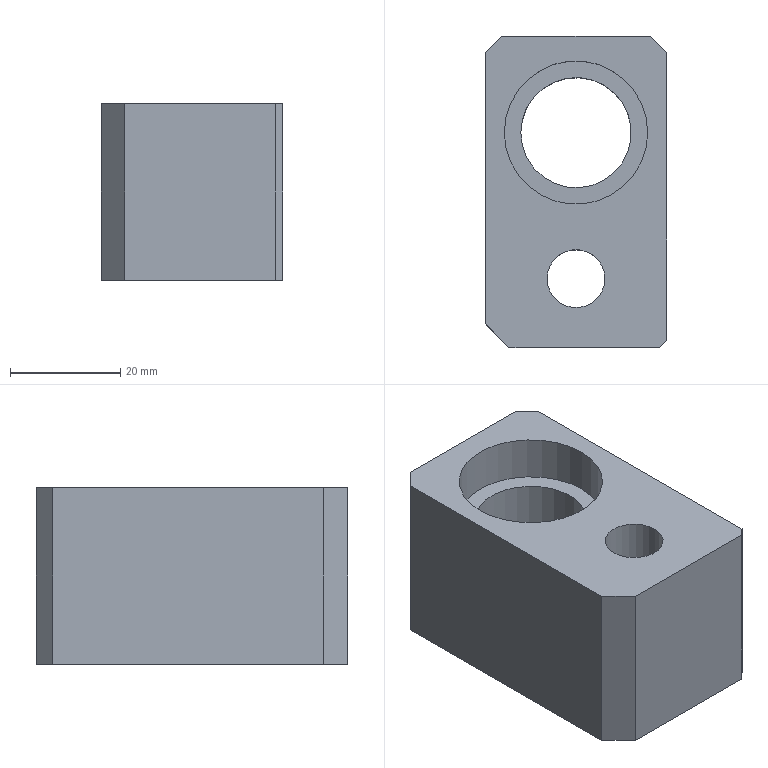Part | STEP file | lll_id2666_x_t | 1 solid | 16 faces | box 33 x 56.5 x 32 mm | volume 42057 mm3 | plane 12 | cylinder 4 | commonest cylinder face diameters 10.5 x1 17 x1 20 x1 26 x1
STEP:
#1=CARTESIAN_POINT('',(427.,300.,60.5));
#2=VERTEX_POINT('',#1);
#3=CARTESIAN_POINT('',(437.,300.,60.5));
#4=DIRECTION('',(0.,0.,1.));
#5=DIRECTION('',(-1.,0.,0.));
#6=AXIS2_PLACEMENT_3D('',#3,#4,#5);
#7=CIRCLE('',#6,10.);
#8=EDGE_CURVE('',#2,#2,#7,.T.);
#9=ORIENTED_EDGE('',*,*,#8,.T.);
#10=EDGE_LOOP('',(#9));
#11=FACE_BOUND('',#10,.T.);
#12=CARTESIAN_POINT('',(450.5,317.5,60.5));
#13=VERTEX_POINT('',#12);
#14=CARTESIAN_POINT('',(423.5,317.5,60.5));
#15=VERTEX_POINT('',#14);
#16=CARTESIAN_POINT('',(437.,317.5,60.5));
#17=DIRECTION('',(-1.,0.,0.));
#18=VECTOR('',#17,1.);
#19=LINE('',#16,#18);
#20=EDGE_CURVE('',#13,#15,#19,.T.);
#21=ORIENTED_EDGE('',*,*,#20,.F.);
#22=CARTESIAN_POINT('',(453.5,314.5,60.5));
#23=VERTEX_POINT('',#22);
#24=CARTESIAN_POINT('',(434.043,333.957,60.5));
#25=DIRECTION('',(0.7071,-0.7071,0.));
#26=VECTOR('',#25,1.);
#27=LINE('',#24,#26);
#28=EDGE_CURVE('',#13,#23,#27,.T.);
#29=ORIENTED_EDGE('',*,*,#28,.T.);
#30=CARTESIAN_POINT('',(453.5,262.343,60.5));
#31=VERTEX_POINT('',#30);
#32=CARTESIAN_POINT('',(453.5,300.,60.5));
#33=DIRECTION('',(0.,1.,0.));
#34=VECTOR('',#33,1.);
#35=LINE('',#32,#34);
#36=EDGE_CURVE('',#31,#23,#35,.T.);
#37=ORIENTED_EDGE('',*,*,#36,.F.);
#38=CARTESIAN_POINT('',(452.157,261.,60.5));
#39=VERTEX_POINT('',#38);
#40=CARTESIAN_POINT('',(409.396,218.239,60.5));
#41=DIRECTION('',(-0.7071,-0.7071,0.));
#42=VECTOR('',#41,1.);
#43=LINE('',#40,#42);
#44=EDGE_CURVE('',#31,#39,#43,.T.);
#45=ORIENTED_EDGE('',*,*,#44,.T.);
#46=CARTESIAN_POINT('',(424.843,261.,60.5));
#47=VERTEX_POINT('',#46);
#48=CARTESIAN_POINT('',(437.,261.,60.5));
#49=DIRECTION('',(1.,0.,0.));
#50=VECTOR('',#49,1.);
#51=LINE('',#48,#50);
#52=EDGE_CURVE('',#47,#39,#51,.T.);
#53=ORIENTED_EDGE('',*,*,#52,.F.);
#54=CARTESIAN_POINT('',(420.5,265.343,60.5));
#55=VERTEX_POINT('',#54);
#56=CARTESIAN_POINT('',(397.964,287.879,60.5));
#57=DIRECTION('',(-0.7071,0.7071,0.));
#58=VECTOR('',#57,1.);
#59=LINE('',#56,#58);
#60=EDGE_CURVE('',#47,#55,#59,.T.);
#61=ORIENTED_EDGE('',*,*,#60,.T.);
#62=CARTESIAN_POINT('',(420.5,314.5,60.5));
#63=VERTEX_POINT('',#62);
#64=CARTESIAN_POINT('',(420.5,300.,60.5));
#65=DIRECTION('',(0.,-1.,0.));
#66=VECTOR('',#65,1.);
#67=LINE('',#64,#66);
#68=EDGE_CURVE('',#63,#55,#67,.T.);
#69=ORIENTED_EDGE('',*,*,#68,.F.);
#70=CARTESIAN_POINT('',(371.817,265.817,60.5));
#71=DIRECTION('',(0.7071,0.7071,0.));
#72=VECTOR('',#71,1.);
#73=LINE('',#70,#72);
#74=EDGE_CURVE('',#63,#15,#73,.T.);
#75=ORIENTED_EDGE('',*,*,#74,.T.);
#76=EDGE_LOOP('',(#21,#29,#37,#45,#53,#61,#69,#75));
#77=FACE_BOUND('',#76,.T.);
#78=CARTESIAN_POINT('',(445.5,273.5,60.5));
#79=VERTEX_POINT('',#78);
#80=CARTESIAN_POINT('',(437.,273.5,60.5));
#81=DIRECTION('',(0.,0.,1.));
#82=DIRECTION('',(1.,0.,0.));
#83=AXIS2_PLACEMENT_3D('',#80,#81,#82);
#84=CIRCLE('',#83,8.5);
#85=EDGE_CURVE('',#79,#79,#84,.T.);
#86=ORIENTED_EDGE('',*,*,#85,.T.);
#87=EDGE_LOOP('',(#86));
#88=FACE_BOUND('',#87,.T.);
#89=CARTESIAN_POINT('',(368.86,268.775,60.5));
#90=DIRECTION('',(0.,0.,1.));
#91=DIRECTION('',(-1.,0.,0.));
#92=AXIS2_PLACEMENT_3D('',#89,#90,#91);
#93=PLANE('',#92);
#94=ADVANCED_FACE('',(#11,#77,#88),#93,.F.);
#95=CARTESIAN_POINT('',(450.,300.,92.5));
#96=VERTEX_POINT('',#95);
#97=CARTESIAN_POINT('',(437.,300.,92.5));
#98=DIRECTION('',(0.,0.,1.));
#99=DIRECTION('',(1.,0.,0.));
#100=AXIS2_PLACEMENT_3D('',#97,#98,#99);
#101=CIRCLE('',#100,13.);
#102=EDGE_CURVE('',#96,#96,#101,.T.);
#103=ORIENTED_EDGE('',*,*,#102,.F.);
#104=EDGE_LOOP('',(#103));
#105=FACE_BOUND('',#104,.T.);
#106=CARTESIAN_POINT('',(442.25,273.5,92.5));
#107=VERTEX_POINT('',#106);
#108=CARTESIAN_POINT('',(437.,273.5,92.5));
#109=DIRECTION('',(0.,0.,1.));
#110=DIRECTION('',(1.,0.,0.));
#111=AXIS2_PLACEMENT_3D('',#108,#109,#110);
#112=CIRCLE('',#111,5.25);
#113=EDGE_CURVE('',#107,#107,#112,.T.);
#114=ORIENTED_EDGE('',*,*,#113,.F.);
#115=EDGE_LOOP('',(#114));
#116=FACE_BOUND('',#115,.T.);
#117=CARTESIAN_POINT('',(453.5,314.5,92.5));
#118=VERTEX_POINT('',#117);
#119=CARTESIAN_POINT('',(453.5,262.343,92.5));
#120=VERTEX_POINT('',#119);
#121=CARTESIAN_POINT('',(453.5,300.,92.5));
#122=DIRECTION('',(0.,-1.,0.));
#123=VECTOR('',#122,1.);
#124=LINE('',#121,#123);
#125=EDGE_CURVE('',#118,#120,#124,.T.);
#126=ORIENTED_EDGE('',*,*,#125,.F.);
#127=CARTESIAN_POINT('',(450.5,317.5,92.5));
#128=VERTEX_POINT('',#127);
#129=CARTESIAN_POINT('',(434.043,333.957,92.5));
#130=DIRECTION('',(-0.7071,0.7071,0.));
#131=VECTOR('',#130,1.);
#132=LINE('',#129,#131);
#133=EDGE_CURVE('',#118,#128,#132,.T.);
#134=ORIENTED_EDGE('',*,*,#133,.T.);
#135=CARTESIAN_POINT('',(423.5,317.5,92.5));
#136=VERTEX_POINT('',#135);
#137=CARTESIAN_POINT('',(437.,317.5,92.5));
#138=DIRECTION('',(1.,0.,0.));
#139=VECTOR('',#138,1.);
#140=LINE('',#137,#139);
#141=EDGE_CURVE('',#136,#128,#140,.T.);
#142=ORIENTED_EDGE('',*,*,#141,.F.);
#143=CARTESIAN_POINT('',(420.5,314.5,92.5));
#144=VERTEX_POINT('',#143);
#145=CARTESIAN_POINT('',(371.817,265.817,92.5));
#146=DIRECTION('',(-0.7071,-0.7071,0.));
#147=VECTOR('',#146,1.);
#148=LINE('',#145,#147);
#149=EDGE_CURVE('',#136,#144,#148,.T.);
#150=ORIENTED_EDGE('',*,*,#149,.T.);
#151=CARTESIAN_POINT('',(420.5,265.343,92.5));
#152=VERTEX_POINT('',#151);
#153=CARTESIAN_POINT('',(420.5,300.,92.5));
#154=DIRECTION('',(0.,1.,0.));
#155=VECTOR('',#154,1.);
#156=LINE('',#153,#155);
#157=EDGE_CURVE('',#152,#144,#156,.T.);
#158=ORIENTED_EDGE('',*,*,#157,.F.);
#159=CARTESIAN_POINT('',(424.843,261.,92.5));
#160=VERTEX_POINT('',#159);
#161=CARTESIAN_POINT('',(397.964,287.879,92.5));
#162=DIRECTION('',(0.7071,-0.7071,0.));
#163=VECTOR('',#162,1.);
#164=LINE('',#161,#163);
#165=EDGE_CURVE('',#152,#160,#164,.T.);
#166=ORIENTED_EDGE('',*,*,#165,.T.);
#167=CARTESIAN_POINT('',(452.157,261.,92.5));
#168=VERTEX_POINT('',#167);
#169=CARTESIAN_POINT('',(437.,261.,92.5));
#170=DIRECTION('',(-1.,0.,0.));
#171=VECTOR('',#170,1.);
#172=LINE('',#169,#171);
#173=EDGE_CURVE('',#168,#160,#172,.T.);
#174=ORIENTED_EDGE('',*,*,#173,.F.);
#175=CARTESIAN_POINT('',(409.396,218.239,92.5));
#176=DIRECTION('',(0.7071,0.7071,0.));
#177=VECTOR('',#176,1.);
#178=LINE('',#175,#177);
#179=EDGE_CURVE('',#168,#120,#178,.T.);
#180=ORIENTED_EDGE('',*,*,#179,.T.);
#181=EDGE_LOOP('',(#126,#134,#142,#150,#158,#166,#174,#180));
#182=FACE_BOUND('',#181,.T.);
#183=CARTESIAN_POINT('',(368.86,268.775,92.5));
#184=DIRECTION('',(0.,0.,1.));
#185=DIRECTION('',(-1.,0.,0.));
#186=AXIS2_PLACEMENT_3D('',#183,#184,#185);
#187=PLANE('',#186);
#188=ADVANCED_FACE('',(#105,#116,#182),#187,.T.);
#189=ORIENTED_EDGE('',*,*,#141,.T.);
#190=CARTESIAN_POINT('',(450.5,317.5,-8.5));
#191=DIRECTION('',(0.,0.,-1.));
#192=VECTOR('',#191,1.);
#193=LINE('',#190,#192);
#194=EDGE_CURVE('',#128,#13,#193,.T.);
#195=ORIENTED_EDGE('',*,*,#194,.T.);
#196=ORIENTED_EDGE('',*,*,#20,.T.);
#197=CARTESIAN_POINT('',(423.5,317.5,-8.5));
#198=DIRECTION('',(0.,0.,1.));
#199=VECTOR('',#198,1.);
#200=LINE('',#197,#199);
#201=EDGE_CURVE('',#15,#136,#200,.T.);
#202=ORIENTED_EDGE('',*,*,#201,.T.);
#203=EDGE_LOOP('',(#189,#195,#196,#202));
#204=FACE_OUTER_BOUND('',#203,.T.);
#205=CARTESIAN_POINT('',(437.,317.5,-8.5));
#206=DIRECTION('',(0.,1.,0.));
#207=DIRECTION('',(0.,0.,-1.));
#208=AXIS2_PLACEMENT_3D('',#205,#206,#207);
#209=PLANE('',#208);
#210=ADVANCED_FACE('',(#204),#209,.T.);
#211=ORIENTED_EDGE('',*,*,#36,.T.);
#212=CARTESIAN_POINT('',(453.5,314.5,-8.5));
#213=DIRECTION('',(0.,0.,1.));
#214=VECTOR('',#213,1.);
#215=LINE('',#212,#214);
#216=EDGE_CURVE('',#23,#118,#215,.T.);
#217=ORIENTED_EDGE('',*,*,#216,.T.);
#218=ORIENTED_EDGE('',*,*,#125,.T.);
#219=CARTESIAN_POINT('',(453.5,262.343,-8.5));
#220=DIRECTION('',(0.,0.,-1.));
#221=VECTOR('',#220,1.);
#222=LINE('',#219,#221);
#223=EDGE_CURVE('',#120,#31,#222,.T.);
#224=ORIENTED_EDGE('',*,*,#223,.T.);
#225=EDGE_LOOP('',(#211,#217,#218,#224));
#226=FACE_OUTER_BOUND('',#225,.T.);
#227=CARTESIAN_POINT('',(453.5,300.,-8.5));
#228=DIRECTION('',(1.,0.,0.));
#229=DIRECTION('',(0.,0.,1.));
#230=AXIS2_PLACEMENT_3D('',#227,#228,#229);
#231=PLANE('',#230);
#232=ADVANCED_FACE('',(#226),#231,.T.);
#233=ORIENTED_EDGE('',*,*,#173,.T.);
#234=CARTESIAN_POINT('',(424.843,261.,-8.5));
#235=DIRECTION('',(0.,0.,-1.));
#236=VECTOR('',#235,1.);
#237=LINE('',#234,#236);
#238=EDGE_CURVE('',#160,#47,#237,.T.);
#239=ORIENTED_EDGE('',*,*,#238,.T.);
#240=ORIENTED_EDGE('',*,*,#52,.T.);
#241=CARTESIAN_POINT('',(452.157,261.,-8.5));
#242=DIRECTION('',(0.,0.,1.));
#243=VECTOR('',#242,1.);
#244=LINE('',#241,#243);
#245=EDGE_CURVE('',#39,#168,#244,.T.);
#246=ORIENTED_EDGE('',*,*,#245,.T.);
#247=EDGE_LOOP('',(#233,#239,#240,#246));
#248=FACE_OUTER_BOUND('',#247,.T.);
#249=CARTESIAN_POINT('',(437.,261.,-8.5));
#250=DIRECTION('',(0.,-1.,0.));
#251=DIRECTION('',(0.,0.,1.));
#252=AXIS2_PLACEMENT_3D('',#249,#250,#251);
#253=PLANE('',#252);
#254=ADVANCED_FACE('',(#248),#253,.T.);
#255=ORIENTED_EDGE('',*,*,#157,.T.);
#256=CARTESIAN_POINT('',(420.5,314.5,-8.5));
#257=DIRECTION('',(0.,0.,-1.));
#258=VECTOR('',#257,1.);
#259=LINE('',#256,#258);
#260=EDGE_CURVE('',#144,#63,#259,.T.);
#261=ORIENTED_EDGE('',*,*,#260,.T.);
#262=ORIENTED_EDGE('',*,*,#68,.T.);
#263=CARTESIAN_POINT('',(420.5,265.343,-8.5));
#264=DIRECTION('',(0.,0.,1.));
#265=VECTOR('',#264,1.);
#266=LINE('',#263,#265);
#267=EDGE_CURVE('',#55,#152,#266,.T.);
#268=ORIENTED_EDGE('',*,*,#267,.T.);
#269=EDGE_LOOP('',(#255,#261,#262,#268));
#270=FACE_OUTER_BOUND('',#269,.T.);
#271=CARTESIAN_POINT('',(420.5,300.,-8.5));
#272=DIRECTION('',(-1.,0.,0.));
#273=DIRECTION('',(0.,0.,-1.));
#274=AXIS2_PLACEMENT_3D('',#271,#272,#273);
#275=PLANE('',#274);
#276=ADVANCED_FACE('',(#270),#275,.T.);
#277=ORIENTED_EDGE('',*,*,#113,.T.);
#278=EDGE_LOOP('',(#277));
#279=FACE_BOUND('',#278,.T.);
#280=CARTESIAN_POINT('',(442.25,273.5,77.5));
#281=VERTEX_POINT('',#280);
#282=CARTESIAN_POINT('',(437.,273.5,77.5));
#283=DIRECTION('',(0.,0.,-1.));
#284=DIRECTION('',(1.,0.,0.));
#285=AXIS2_PLACEMENT_3D('',#282,#283,#284);
#286=CIRCLE('',#285,5.25);
#287=EDGE_CURVE('',#281,#281,#286,.T.);
#288=ORIENTED_EDGE('',*,*,#287,.T.);
#289=EDGE_LOOP('',(#288));
#290=FACE_BOUND('',#289,.T.);
#291=CARTESIAN_POINT('',(437.,273.5,160.5));
#292=DIRECTION('',(0.,0.,1.));
#293=DIRECTION('',(-1.,0.,0.));
#294=AXIS2_PLACEMENT_3D('',#291,#292,#293);
#295=CYLINDRICAL_SURFACE('',#294,5.25);
#296=ADVANCED_FACE('',(#279,#290),#295,.F.);
#297=ORIENTED_EDGE('',*,*,#287,.F.);
#298=EDGE_LOOP('',(#297));
#299=FACE_BOUND('',#298,.T.);
#300=CARTESIAN_POINT('',(445.5,273.5,77.5));
#301=VERTEX_POINT('',#300);
#302=CARTESIAN_POINT('',(437.,273.5,77.5));
#303=DIRECTION('',(0.,0.,-1.));
#304=DIRECTION('',(1.,0.,0.));
#305=AXIS2_PLACEMENT_3D('',#302,#303,#304);
#306=CIRCLE('',#305,8.5);
#307=EDGE_CURVE('',#301,#301,#306,.T.);
#308=ORIENTED_EDGE('',*,*,#307,.T.);
#309=EDGE_LOOP('',(#308));
#310=FACE_BOUND('',#309,.T.);
#311=CARTESIAN_POINT('',(437.,273.5,77.5));
#312=DIRECTION('',(0.,0.,1.));
#313=DIRECTION('',(-1.,0.,0.));
#314=AXIS2_PLACEMENT_3D('',#311,#312,#313);
#315=PLANE('',#314);
#316=ADVANCED_FACE('',(#299,#310),#315,.F.);
#317=ORIENTED_EDGE('',*,*,#307,.F.);
#318=EDGE_LOOP('',(#317));
#319=FACE_BOUND('',#318,.T.);
#320=ORIENTED_EDGE('',*,*,#85,.F.);
#321=EDGE_LOOP('',(#320));
#322=FACE_BOUND('',#321,.T.);
#323=CARTESIAN_POINT('',(437.,273.5,60.5));
#324=DIRECTION('',(0.,0.,1.));
#325=DIRECTION('',(-1.,0.,0.));
#326=AXIS2_PLACEMENT_3D('',#323,#324,#325);
#327=CYLINDRICAL_SURFACE('',#326,8.5);
#328=ADVANCED_FACE('',(#319,#322),#327,.F.);
#329=ORIENTED_EDGE('',*,*,#44,.F.);
#330=ORIENTED_EDGE('',*,*,#223,.F.);
#331=ORIENTED_EDGE('',*,*,#179,.F.);
#332=ORIENTED_EDGE('',*,*,#245,.F.);
#333=EDGE_LOOP('',(#329,#330,#331,#332));
#334=FACE_OUTER_BOUND('',#333,.T.);
#335=CARTESIAN_POINT('',(449.328,258.172,-8.5));
#336=DIRECTION('',(-0.7071,0.7071,0.));
#337=DIRECTION('',(0.,0.,1.));
#338=AXIS2_PLACEMENT_3D('',#335,#336,#337);
#339=PLANE('',#338);
#340=ADVANCED_FACE('',(#334),#339,.F.);
#341=ORIENTED_EDGE('',*,*,#165,.F.);
#342=ORIENTED_EDGE('',*,*,#267,.F.);
#343=ORIENTED_EDGE('',*,*,#60,.F.);
#344=ORIENTED_EDGE('',*,*,#238,.F.);
#345=EDGE_LOOP('',(#341,#342,#343,#344));
#346=FACE_OUTER_BOUND('',#345,.T.);
#347=CARTESIAN_POINT('',(427.672,258.172,-8.5));
#348=DIRECTION('',(0.7071,0.7071,0.));
#349=DIRECTION('',(0.,0.,-1.));
#350=AXIS2_PLACEMENT_3D('',#347,#348,#349);
#351=PLANE('',#350);
#352=ADVANCED_FACE('',(#346),#351,.F.);
#353=ORIENTED_EDGE('',*,*,#8,.F.);
#354=EDGE_LOOP('',(#353));
#355=FACE_BOUND('',#354,.T.);
#356=CARTESIAN_POINT('',(427.,300.,84.3));
#357=VERTEX_POINT('',#356);
#358=CARTESIAN_POINT('',(437.,300.,84.3));
#359=DIRECTION('',(0.,0.,-1.));
#360=DIRECTION('',(1.,0.,0.));
#361=AXIS2_PLACEMENT_3D('',#358,#359,#360);
#362=CIRCLE('',#361,10.);
#363=EDGE_CURVE('',#357,#357,#362,.T.);
#364=ORIENTED_EDGE('',*,*,#363,.F.);
#365=EDGE_LOOP('',(#364));
#366=FACE_BOUND('',#365,.T.);
#367=CARTESIAN_POINT('',(437.,300.,124.8));
#368=DIRECTION('',(0.,0.,-1.));
#369=DIRECTION('',(1.,0.,0.));
#370=AXIS2_PLACEMENT_3D('',#367,#368,#369);
#371=CYLINDRICAL_SURFACE('',#370,10.);
#372=ADVANCED_FACE('',(#355,#366),#371,.F.);
#373=CARTESIAN_POINT('',(450.,300.,84.3));
#374=VERTEX_POINT('',#373);
#375=CARTESIAN_POINT('',(437.,300.,84.3));
#376=DIRECTION('',(0.,0.,1.));
#377=DIRECTION('',(1.,0.,0.));
#378=AXIS2_PLACEMENT_3D('',#375,#376,#377);
#379=CIRCLE('',#378,13.);
#380=EDGE_CURVE('',#374,#374,#379,.T.);
#381=ORIENTED_EDGE('',*,*,#380,.T.);
#382=EDGE_LOOP('',(#381));
#383=FACE_BOUND('',#382,.T.);
#384=ORIENTED_EDGE('',*,*,#363,.T.);
#385=EDGE_LOOP('',(#384));
#386=FACE_BOUND('',#385,.T.);
#387=CARTESIAN_POINT('',(437.,300.,84.3));
#388=DIRECTION('',(0.,0.,1.));
#389=DIRECTION('',(-1.,0.,0.));
#390=AXIS2_PLACEMENT_3D('',#387,#388,#389);
#391=PLANE('',#390);
#392=ADVANCED_FACE('',(#383,#386),#391,.T.);
#393=ORIENTED_EDGE('',*,*,#380,.F.);
#394=EDGE_LOOP('',(#393));
#395=FACE_BOUND('',#394,.T.);
#396=ORIENTED_EDGE('',*,*,#102,.T.);
#397=EDGE_LOOP('',(#396));
#398=FACE_BOUND('',#397,.T.);
#399=CARTESIAN_POINT('',(437.,300.,124.8));
#400=DIRECTION('',(0.,0.,-1.));
#401=DIRECTION('',(1.,0.,0.));
#402=AXIS2_PLACEMENT_3D('',#399,#400,#401);
#403=CYLINDRICAL_SURFACE('',#402,13.);
#404=ADVANCED_FACE('',(#395,#398),#403,.F.);
#405=ORIENTED_EDGE('',*,*,#28,.F.);
#406=ORIENTED_EDGE('',*,*,#194,.F.);
#407=ORIENTED_EDGE('',*,*,#133,.F.);
#408=ORIENTED_EDGE('',*,*,#216,.F.);
#409=EDGE_LOOP('',(#405,#406,#407,#408));
#410=FACE_OUTER_BOUND('',#409,.T.);
#411=CARTESIAN_POINT('',(453.5,314.5,-8.5));
#412=DIRECTION('',(-0.7071,-0.7071,0.));
#413=DIRECTION('',(0.,0.,1.));
#414=AXIS2_PLACEMENT_3D('',#411,#412,#413);
#415=PLANE('',#414);
#416=ADVANCED_FACE('',(#410),#415,.F.);
#417=ORIENTED_EDGE('',*,*,#74,.F.);
#418=ORIENTED_EDGE('',*,*,#260,.F.);
#419=ORIENTED_EDGE('',*,*,#149,.F.);
#420=ORIENTED_EDGE('',*,*,#201,.F.);
#421=EDGE_LOOP('',(#417,#418,#419,#420));
#422=FACE_OUTER_BOUND('',#421,.T.);
#423=CARTESIAN_POINT('',(423.5,317.5,-8.5));
#424=DIRECTION('',(0.7071,-0.7071,0.));
#425=DIRECTION('',(0.,0.,1.));
#426=AXIS2_PLACEMENT_3D('',#423,#424,#425);
#427=PLANE('',#426);
#428=ADVANCED_FACE('',(#422),#427,.F.);
#429=CLOSED_SHELL('',(#94,#188,#210,#232,#254,#276,#296,#316,#328,#340,#352,#372,#392,#404,#416,#428));
#430=MANIFOLD_SOLID_BREP('',#429);
#431=(LENGTH_UNIT()NAMED_UNIT(*)SI_UNIT(.MILLI.,.METRE.));
#432=UNCERTAINTY_MEASURE_WITH_UNIT(LENGTH_MEASURE(0.00002),#431,'','');
#433=(NAMED_UNIT(*)PLANE_ANGLE_UNIT()SI_UNIT($,.RADIAN.));
#434=PLANE_ANGLE_MEASURE_WITH_UNIT(PLANE_ANGLE_MEASURE(0.01745),#433);
#435=DIMENSIONAL_EXPONENTS(0.,0.,0.,0.,0.,0.,0.);
#436=(CONVERSION_BASED_UNIT('DEGREE',#434)NAMED_UNIT(#435)PLANE_ANGLE_UNIT());
#437=(NAMED_UNIT(*)SI_UNIT($,.STERADIAN.)SOLID_ANGLE_UNIT());
#438=(GEOMETRIC_REPRESENTATION_CONTEXT(3)GLOBAL_UNCERTAINTY_ASSIGNED_CONTEXT((#432))GLOBAL_UNIT_ASSIGNED_CONTEXT((#431,#436,#437))REPRESENTATION_CONTEXT('',''));
#439=ADVANCED_BREP_SHAPE_REPRESENTATION('',(#430),#438);